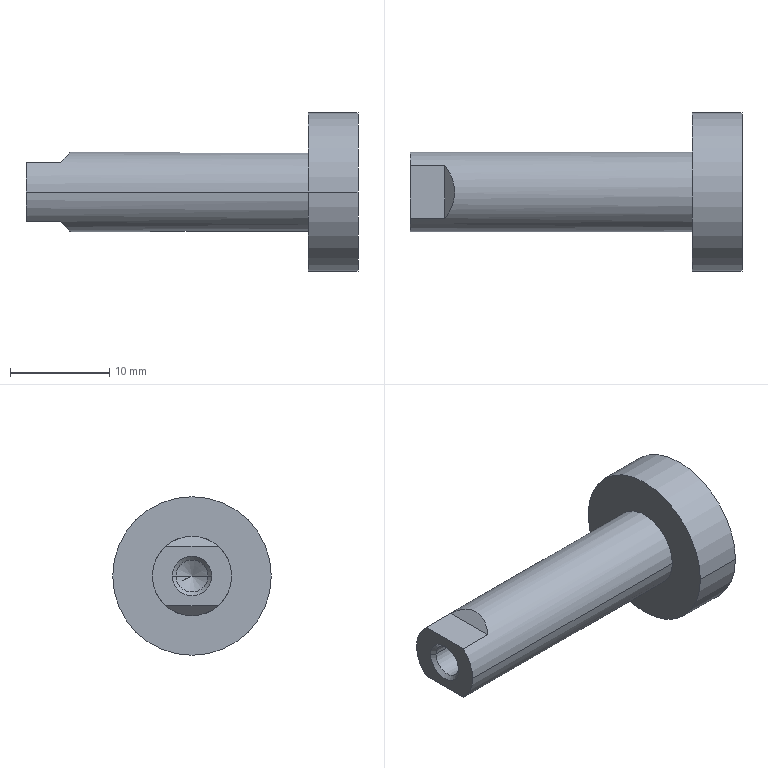Part | SolidWorks | features RefAxis 3, 3DProfileFeature 1, ICE 1, Revolution 1 | 1 solid | 17 faces | box 33.5 x 16 x 16 mm | volume 2340 mm3 | plane 7 | cylinder 6 | cone 4 | commonest cylinder face diameters 3.242 x2 8 x2 16 x2
STEP:
#1=CARTESIAN_POINT('',(30.,-8.,0.));
#2=VERTEX_POINT('',#1);
#3=CARTESIAN_POINT('',(30.,8.,0.));
#4=VERTEX_POINT('',#3);
#5=CARTESIAN_POINT('',(30.,0.,0.));
#6=DIRECTION('',(-1.,0.,0.));
#7=DIRECTION('',(0.,-1.,0.));
#8=AXIS2_PLACEMENT_3D('',#5,#6,#7);
#9=CIRCLE('',#8,8.);
#10=EDGE_CURVE('',#2,#4,#9,.T.);
#11=ORIENTED_EDGE('',*,*,#10,.T.);
#12=CARTESIAN_POINT('',(25.,8.,0.));
#13=VERTEX_POINT('',#12);
#14=CARTESIAN_POINT('',(30.,8.,0.));
#15=DIRECTION('',(-1.,0.,0.));
#16=VECTOR('',#15,1000.);
#17=LINE('',#14,#16);
#18=EDGE_CURVE('',#4,#13,#17,.T.);
#19=ORIENTED_EDGE('',*,*,#18,.T.);
#20=CARTESIAN_POINT('',(25.,-8.,0.));
#21=VERTEX_POINT('',#20);
#22=CARTESIAN_POINT('',(25.,0.,0.));
#23=DIRECTION('',(-1.,0.,0.));
#24=DIRECTION('',(0.,-1.,0.));
#25=AXIS2_PLACEMENT_3D('',#22,#23,#24);
#26=CIRCLE('',#25,8.);
#27=EDGE_CURVE('',#21,#13,#26,.T.);
#28=ORIENTED_EDGE('',*,*,#27,.F.);
#29=CARTESIAN_POINT('',(30.,-8.,0.));
#30=DIRECTION('',(-1.,0.,0.));
#31=VECTOR('',#30,1000.);
#32=LINE('',#29,#31);
#33=EDGE_CURVE('',#2,#21,#32,.T.);
#34=ORIENTED_EDGE('',*,*,#33,.F.);
#35=EDGE_LOOP('',(#11,#19,#28,#34));
#36=FACE_OUTER_BOUND('',#35,.T.);
#37=CARTESIAN_POINT('',(30.,0.,0.));
#38=DIRECTION('',(-1.,0.,0.));
#39=DIRECTION('',(0.,-1.,0.));
#40=AXIS2_PLACEMENT_3D('',#37,#38,#39);
#41=CYLINDRICAL_SURFACE('',#40,8.);
#42=ADVANCED_FACE('',(#36),#41,.T.);
#43=CARTESIAN_POINT('',(25.,-4.,0.));
#44=VERTEX_POINT('',#43);
#45=CARTESIAN_POINT('',(25.,4.,0.));
#46=VERTEX_POINT('',#45);
#47=CARTESIAN_POINT('',(25.,0.,0.));
#48=DIRECTION('',(-1.,0.,0.));
#49=DIRECTION('',(0.,-1.,0.));
#50=AXIS2_PLACEMENT_3D('',#47,#48,#49);
#51=CIRCLE('',#50,4.);
#52=EDGE_CURVE('',#44,#46,#51,.T.);
#53=ORIENTED_EDGE('',*,*,#52,.T.);
#54=CARTESIAN_POINT('',(-3.5,4.,0.));
#55=VERTEX_POINT('',#54);
#56=CARTESIAN_POINT('',(30.,4.,0.));
#57=DIRECTION('',(-1.,0.,0.));
#58=VECTOR('',#57,1000.);
#59=LINE('',#56,#58);
#60=EDGE_CURVE('',#46,#55,#59,.T.);
#61=ORIENTED_EDGE('',*,*,#60,.T.);
#62=CARTESIAN_POINT('',(-3.5,2.646,3.));
#63=VERTEX_POINT('',#62);
#64=CARTESIAN_POINT('',(-3.5,0.,0.));
#65=DIRECTION('',(-1.,0.,0.));
#66=DIRECTION('',(0.,-1.,0.));
#67=AXIS2_PLACEMENT_3D('',#64,#65,#66);
#68=CIRCLE('',#67,4.);
#69=EDGE_CURVE('',#63,#55,#68,.T.);
#70=ORIENTED_EDGE('',*,*,#69,.F.);
#71=CARTESIAN_POINT('',(0.,2.646,3.));
#72=VERTEX_POINT('',#71);
#73=CARTESIAN_POINT('',(30.,2.646,3.));
#74=DIRECTION('',(1.,0.,0.));
#75=VECTOR('',#74,1000.);
#76=LINE('',#73,#75);
#77=EDGE_CURVE('',#63,#72,#76,.T.);
#78=ORIENTED_EDGE('',*,*,#77,.T.);
#79=CARTESIAN_POINT('',(0.,-2.646,3.));
#80=VERTEX_POINT('',#79);
#81=CARTESIAN_POINT('',(0.,2.646,3.));
#82=CARTESIAN_POINT('',(1.4,1.058,4.4));
#83=CARTESIAN_POINT('',(1.4,-1.058,4.4));
#84=CARTESIAN_POINT('',(0.,-2.646,3.));
#85=(BOUNDED_CURVE()B_SPLINE_CURVE(3,(#81,#82,#83,#84),.UNSPECIFIED.,.F.,.T.)B_SPLINE_CURVE_WITH_KNOTS((4,4),(2.419,3.864),.UNSPECIFIED.)CURVE()GEOMETRIC_REPRESENTATION_ITEM()RATIONAL_B_SPLINE_CURVE((1.,0.8333,0.8333,1.))REPRESENTATION_ITEM(''));
#86=EDGE_CURVE('',#72,#80,#85,.T.);
#87=ORIENTED_EDGE('',*,*,#86,.T.);
#88=CARTESIAN_POINT('',(-3.5,-2.646,3.));
#89=VERTEX_POINT('',#88);
#90=CARTESIAN_POINT('',(30.,-2.646,3.));
#91=DIRECTION('',(-1.,0.,0.));
#92=VECTOR('',#91,1000.);
#93=LINE('',#90,#92);
#94=EDGE_CURVE('',#80,#89,#93,.T.);
#95=ORIENTED_EDGE('',*,*,#94,.T.);
#96=CARTESIAN_POINT('',(-3.5,-4.,0.));
#97=VERTEX_POINT('',#96);
#98=CARTESIAN_POINT('',(-3.5,0.,0.));
#99=DIRECTION('',(-1.,0.,0.));
#100=DIRECTION('',(0.,-1.,0.));
#101=AXIS2_PLACEMENT_3D('',#98,#99,#100);
#102=CIRCLE('',#101,4.);
#103=EDGE_CURVE('',#97,#89,#102,.T.);
#104=ORIENTED_EDGE('',*,*,#103,.F.);
#105=CARTESIAN_POINT('',(30.,-4.,0.));
#106=DIRECTION('',(-1.,0.,0.));
#107=VECTOR('',#106,1000.);
#108=LINE('',#105,#107);
#109=EDGE_CURVE('',#44,#97,#108,.T.);
#110=ORIENTED_EDGE('',*,*,#109,.F.);
#111=EDGE_LOOP('',(#53,#61,#70,#78,#87,#95,#104,#110));
#112=FACE_OUTER_BOUND('',#111,.T.);
#113=CARTESIAN_POINT('',(30.,0.,0.));
#114=DIRECTION('',(-1.,0.,0.));
#115=DIRECTION('',(0.,-1.,0.));
#116=AXIS2_PLACEMENT_3D('',#113,#114,#115);
#117=CYLINDRICAL_SURFACE('',#116,4.);
#118=ADVANCED_FACE('',(#112),#117,.T.);
#119=CARTESIAN_POINT('',(-3.121,1.621,0.));
#120=VERTEX_POINT('',#119);
#121=CARTESIAN_POINT('',(-3.121,-1.621,0.));
#122=VERTEX_POINT('',#121);
#123=CARTESIAN_POINT('',(-3.121,0.,0.));
#124=DIRECTION('',(-1.,0.,0.));
#125=DIRECTION('',(0.,-1.,0.));
#126=AXIS2_PLACEMENT_3D('',#123,#124,#125);
#127=CIRCLE('',#126,1.621);
#128=EDGE_CURVE('',#120,#122,#127,.T.);
#129=ORIENTED_EDGE('',*,*,#128,.F.);
#130=CARTESIAN_POINT('',(-3.5,2.,0.));
#131=VERTEX_POINT('',#130);
#132=CARTESIAN_POINT('',(-3.5,2.,0.));
#133=DIRECTION('',(-0.7071,0.7071,0.));
#134=VECTOR('',#133,1000.);
#135=LINE('',#132,#134);
#136=EDGE_CURVE('',#120,#131,#135,.T.);
#137=ORIENTED_EDGE('',*,*,#136,.T.);
#138=CARTESIAN_POINT('',(-3.5,-2.,0.));
#139=VERTEX_POINT('',#138);
#140=CARTESIAN_POINT('',(-3.5,0.,0.));
#141=DIRECTION('',(-1.,0.,0.));
#142=DIRECTION('',(0.,-1.,0.));
#143=AXIS2_PLACEMENT_3D('',#140,#141,#142);
#144=CIRCLE('',#143,2.);
#145=EDGE_CURVE('',#131,#139,#144,.T.);
#146=ORIENTED_EDGE('',*,*,#145,.T.);
#147=CARTESIAN_POINT('',(-3.5,-2.,0.));
#148=DIRECTION('',(-0.7071,-0.7071,0.));
#149=VECTOR('',#148,1000.);
#150=LINE('',#147,#149);
#151=EDGE_CURVE('',#122,#139,#150,.T.);
#152=ORIENTED_EDGE('',*,*,#151,.F.);
#153=EDGE_LOOP('',(#129,#137,#146,#152));
#154=FACE_OUTER_BOUND('',#153,.T.);
#155=CARTESIAN_POINT('',(-3.5,0.,0.));
#156=DIRECTION('',(-1.,0.,0.));
#157=DIRECTION('',(0.,-1.,0.));
#158=AXIS2_PLACEMENT_3D('',#155,#156,#157);
#159=CONICAL_SURFACE('',#158,2.,0.7854);
#160=ADVANCED_FACE('',(#154),#159,.F.);
#161=CARTESIAN_POINT('',(4.5,1.621,0.));
#162=VERTEX_POINT('',#161);
#163=CARTESIAN_POINT('',(4.5,-1.621,0.));
#164=VERTEX_POINT('',#163);
#165=CARTESIAN_POINT('',(4.5,0.,0.));
#166=DIRECTION('',(-1.,0.,0.));
#167=DIRECTION('',(0.,-1.,0.));
#168=AXIS2_PLACEMENT_3D('',#165,#166,#167);
#169=CIRCLE('',#168,1.621);
#170=EDGE_CURVE('',#162,#164,#169,.T.);
#171=ORIENTED_EDGE('',*,*,#170,.F.);
#172=CARTESIAN_POINT('',(30.,1.621,0.));
#173=DIRECTION('',(-1.,0.,0.));
#174=VECTOR('',#173,1000.);
#175=LINE('',#172,#174);
#176=EDGE_CURVE('',#162,#120,#175,.T.);
#177=ORIENTED_EDGE('',*,*,#176,.T.);
#178=ORIENTED_EDGE('',*,*,#128,.T.);
#179=CARTESIAN_POINT('',(30.,-1.621,0.));
#180=DIRECTION('',(-1.,0.,0.));
#181=VECTOR('',#180,1000.);
#182=LINE('',#179,#181);
#183=EDGE_CURVE('',#164,#122,#182,.T.);
#184=ORIENTED_EDGE('',*,*,#183,.F.);
#185=EDGE_LOOP('',(#171,#177,#178,#184));
#186=FACE_OUTER_BOUND('',#185,.T.);
#187=CARTESIAN_POINT('',(30.,0.,0.));
#188=DIRECTION('',(-1.,0.,0.));
#189=DIRECTION('',(0.,-1.,0.));
#190=AXIS2_PLACEMENT_3D('',#187,#188,#189);
#191=CYLINDRICAL_SURFACE('',#190,1.621);
#192=ADVANCED_FACE('',(#186),#191,.F.);
#193=CARTESIAN_POINT('',(5.436,0.,0.));
#194=VERTEX_POINT('',#193);
#195=CARTESIAN_POINT('',(4.5,-1.621,0.));
#196=DIRECTION('',(-0.5,-0.866,0.));
#197=VECTOR('',#196,1000.);
#198=LINE('',#195,#197);
#199=EDGE_CURVE('',#194,#164,#198,.T.);
#200=ORIENTED_EDGE('',*,*,#199,.F.);
#201=CARTESIAN_POINT('',(4.5,1.621,0.));
#202=DIRECTION('',(-0.5,0.866,0.));
#203=VECTOR('',#202,1000.);
#204=LINE('',#201,#203);
#205=EDGE_CURVE('',#194,#162,#204,.T.);
#206=ORIENTED_EDGE('',*,*,#205,.T.);
#207=ORIENTED_EDGE('',*,*,#170,.T.);
#208=EDGE_LOOP('',(#200,#206,#207));
#209=FACE_OUTER_BOUND('',#208,.T.);
#210=CARTESIAN_POINT('',(4.5,0.,0.));
#211=DIRECTION('',(-1.,0.,0.));
#212=DIRECTION('',(0.,-1.,0.));
#213=AXIS2_PLACEMENT_3D('',#210,#211,#212);
#214=CONICAL_SURFACE('',#213,1.621,1.047);
#215=ADVANCED_FACE('',(#209),#214,.F.);
#216=ORIENTED_EDGE('',*,*,#205,.F.);
#217=ORIENTED_EDGE('',*,*,#199,.T.);
#218=CARTESIAN_POINT('',(4.5,0.,0.));
#219=DIRECTION('',(-1.,0.,0.));
#220=DIRECTION('',(0.,-1.,0.));
#221=AXIS2_PLACEMENT_3D('',#218,#219,#220);
#222=CIRCLE('',#221,1.621);
#223=EDGE_CURVE('',#164,#162,#222,.T.);
#224=ORIENTED_EDGE('',*,*,#223,.T.);
#225=EDGE_LOOP('',(#216,#217,#224));
#226=FACE_OUTER_BOUND('',#225,.T.);
#227=CARTESIAN_POINT('',(4.5,0.,0.));
#228=DIRECTION('',(-1.,0.,0.));
#229=DIRECTION('',(0.,-1.,0.));
#230=AXIS2_PLACEMENT_3D('',#227,#228,#229);
#231=CONICAL_SURFACE('',#230,1.621,1.047);
#232=ADVANCED_FACE('',(#226),#231,.F.);
#233=ORIENTED_EDGE('',*,*,#176,.F.);
#234=ORIENTED_EDGE('',*,*,#223,.F.);
#235=ORIENTED_EDGE('',*,*,#183,.T.);
#236=CARTESIAN_POINT('',(-3.121,0.,0.));
#237=DIRECTION('',(-1.,0.,0.));
#238=DIRECTION('',(0.,-1.,0.));
#239=AXIS2_PLACEMENT_3D('',#236,#237,#238);
#240=CIRCLE('',#239,1.621);
#241=EDGE_CURVE('',#122,#120,#240,.T.);
#242=ORIENTED_EDGE('',*,*,#241,.T.);
#243=EDGE_LOOP('',(#233,#234,#235,#242));
#244=FACE_OUTER_BOUND('',#243,.T.);
#245=CARTESIAN_POINT('',(30.,0.,0.));
#246=DIRECTION('',(-1.,0.,0.));
#247=DIRECTION('',(0.,-1.,0.));
#248=AXIS2_PLACEMENT_3D('',#245,#246,#247);
#249=CYLINDRICAL_SURFACE('',#248,1.621);
#250=ADVANCED_FACE('',(#244),#249,.F.);
#251=ORIENTED_EDGE('',*,*,#136,.F.);
#252=ORIENTED_EDGE('',*,*,#241,.F.);
#253=ORIENTED_EDGE('',*,*,#151,.T.);
#254=CARTESIAN_POINT('',(-3.5,0.,0.));
#255=DIRECTION('',(-1.,0.,0.));
#256=DIRECTION('',(0.,-1.,0.));
#257=AXIS2_PLACEMENT_3D('',#254,#255,#256);
#258=CIRCLE('',#257,2.);
#259=EDGE_CURVE('',#139,#131,#258,.T.);
#260=ORIENTED_EDGE('',*,*,#259,.T.);
#261=EDGE_LOOP('',(#251,#252,#253,#260));
#262=FACE_OUTER_BOUND('',#261,.T.);
#263=CARTESIAN_POINT('',(-3.5,0.,0.));
#264=DIRECTION('',(-1.,0.,0.));
#265=DIRECTION('',(0.,-1.,0.));
#266=AXIS2_PLACEMENT_3D('',#263,#264,#265);
#267=CONICAL_SURFACE('',#266,2.,0.7854);
#268=ADVANCED_FACE('',(#262),#267,.F.);
#269=ORIENTED_EDGE('',*,*,#259,.F.);
#270=ORIENTED_EDGE('',*,*,#145,.F.);
#271=EDGE_LOOP('',(#269,#270));
#272=FACE_BOUND('',#271,.T.);
#273=ORIENTED_EDGE('',*,*,#69,.T.);
#274=CARTESIAN_POINT('',(-3.5,2.646,-3.));
#275=VERTEX_POINT('',#274);
#276=CARTESIAN_POINT('',(-3.5,0.,0.));
#277=DIRECTION('',(-1.,0.,0.));
#278=DIRECTION('',(0.,-1.,0.));
#279=AXIS2_PLACEMENT_3D('',#276,#277,#278);
#280=CIRCLE('',#279,4.);
#281=EDGE_CURVE('',#55,#275,#280,.T.);
#282=ORIENTED_EDGE('',*,*,#281,.T.);
#283=CARTESIAN_POINT('',(-3.5,-2.646,-3.));
#284=VERTEX_POINT('',#283);
#285=CARTESIAN_POINT('',(-3.5,-8.,-3.));
#286=DIRECTION('',(0.,1.,0.));
#287=VECTOR('',#286,1000.);
#288=LINE('',#285,#287);
#289=EDGE_CURVE('',#284,#275,#288,.T.);
#290=ORIENTED_EDGE('',*,*,#289,.F.);
#291=CARTESIAN_POINT('',(-3.5,0.,0.));
#292=DIRECTION('',(-1.,0.,0.));
#293=DIRECTION('',(0.,-1.,0.));
#294=AXIS2_PLACEMENT_3D('',#291,#292,#293);
#295=CIRCLE('',#294,4.);
#296=EDGE_CURVE('',#284,#97,#295,.T.);
#297=ORIENTED_EDGE('',*,*,#296,.T.);
#298=ORIENTED_EDGE('',*,*,#103,.T.);
#299=CARTESIAN_POINT('',(-3.5,-8.,3.));
#300=DIRECTION('',(0.,1.,0.));
#301=VECTOR('',#300,1000.);
#302=LINE('',#299,#301);
#303=EDGE_CURVE('',#89,#63,#302,.T.);
#304=ORIENTED_EDGE('',*,*,#303,.T.);
#305=EDGE_LOOP('',(#273,#282,#290,#297,#298,#304));
#306=FACE_OUTER_BOUND('',#305,.T.);
#307=CARTESIAN_POINT('',(-3.5,2.,0.));
#308=DIRECTION('',(1.,0.,0.));
#309=DIRECTION('',(0.,1.,0.));
#310=AXIS2_PLACEMENT_3D('',#307,#308,#309);
#311=PLANE('',#310);
#312=ADVANCED_FACE('',(#272,#306),#311,.F.);
#313=ORIENTED_EDGE('',*,*,#60,.F.);
#314=CARTESIAN_POINT('',(25.,0.,0.));
#315=DIRECTION('',(-1.,0.,0.));
#316=DIRECTION('',(0.,-1.,0.));
#317=AXIS2_PLACEMENT_3D('',#314,#315,#316);
#318=CIRCLE('',#317,4.);
#319=EDGE_CURVE('',#46,#44,#318,.T.);
#320=ORIENTED_EDGE('',*,*,#319,.T.);
#321=ORIENTED_EDGE('',*,*,#109,.T.);
#322=ORIENTED_EDGE('',*,*,#296,.F.);
#323=CARTESIAN_POINT('',(0.,-2.646,-3.));
#324=VERTEX_POINT('',#323);
#325=CARTESIAN_POINT('',(30.,-2.646,-3.));
#326=DIRECTION('',(1.,0.,0.));
#327=VECTOR('',#326,1000.);
#328=LINE('',#325,#327);
#329=EDGE_CURVE('',#284,#324,#328,.T.);
#330=ORIENTED_EDGE('',*,*,#329,.T.);
#331=CARTESIAN_POINT('',(0.,2.646,-3.));
#332=VERTEX_POINT('',#331);
#333=CARTESIAN_POINT('',(0.,-2.646,-3.));
#334=CARTESIAN_POINT('',(1.4,-1.058,-4.4));
#335=CARTESIAN_POINT('',(1.4,1.058,-4.4));
#336=CARTESIAN_POINT('',(0.,2.646,-3.));
#337=(BOUNDED_CURVE()B_SPLINE_CURVE(3,(#333,#334,#335,#336),.UNSPECIFIED.,.F.,.F.)B_SPLINE_CURVE_WITH_KNOTS((4,4),(2.419,3.864),.UNSPECIFIED.)CURVE()GEOMETRIC_REPRESENTATION_ITEM()RATIONAL_B_SPLINE_CURVE((1.,0.8333,0.8333,1.))REPRESENTATION_ITEM(''));
#338=EDGE_CURVE('',#324,#332,#337,.T.);
#339=ORIENTED_EDGE('',*,*,#338,.T.);
#340=CARTESIAN_POINT('',(30.,2.646,-3.));
#341=DIRECTION('',(-1.,0.,0.));
#342=VECTOR('',#341,1000.);
#343=LINE('',#340,#342);
#344=EDGE_CURVE('',#332,#275,#343,.T.);
#345=ORIENTED_EDGE('',*,*,#344,.T.);
#346=ORIENTED_EDGE('',*,*,#281,.F.);
#347=EDGE_LOOP('',(#313,#320,#321,#322,#330,#339,#345,#346));
#348=FACE_OUTER_BOUND('',#347,.T.);
#349=CARTESIAN_POINT('',(30.,0.,0.));
#350=DIRECTION('',(-1.,0.,0.));
#351=DIRECTION('',(0.,-1.,0.));
#352=AXIS2_PLACEMENT_3D('',#349,#350,#351);
#353=CYLINDRICAL_SURFACE('',#352,4.);
#354=ADVANCED_FACE('',(#348),#353,.T.);
#355=ORIENTED_EDGE('',*,*,#52,.F.);
#356=ORIENTED_EDGE('',*,*,#319,.F.);
#357=EDGE_LOOP('',(#355,#356));
#358=FACE_BOUND('',#357,.T.);
#359=ORIENTED_EDGE('',*,*,#27,.T.);
#360=CARTESIAN_POINT('',(25.,0.,0.));
#361=DIRECTION('',(-1.,0.,0.));
#362=DIRECTION('',(0.,-1.,0.));
#363=AXIS2_PLACEMENT_3D('',#360,#361,#362);
#364=CIRCLE('',#363,8.);
#365=EDGE_CURVE('',#13,#21,#364,.T.);
#366=ORIENTED_EDGE('',*,*,#365,.T.);
#367=EDGE_LOOP('',(#359,#366));
#368=FACE_OUTER_BOUND('',#367,.T.);
#369=CARTESIAN_POINT('',(25.,4.,0.));
#370=DIRECTION('',(1.,0.,0.));
#371=DIRECTION('',(0.,1.,0.));
#372=AXIS2_PLACEMENT_3D('',#369,#370,#371);
#373=PLANE('',#372);
#374=ADVANCED_FACE('',(#358,#368),#373,.F.);
#375=ORIENTED_EDGE('',*,*,#18,.F.);
#376=CARTESIAN_POINT('',(30.,0.,0.));
#377=DIRECTION('',(-1.,0.,0.));
#378=DIRECTION('',(0.,-1.,0.));
#379=AXIS2_PLACEMENT_3D('',#376,#377,#378);
#380=CIRCLE('',#379,8.);
#381=EDGE_CURVE('',#4,#2,#380,.T.);
#382=ORIENTED_EDGE('',*,*,#381,.T.);
#383=ORIENTED_EDGE('',*,*,#33,.T.);
#384=ORIENTED_EDGE('',*,*,#365,.F.);
#385=EDGE_LOOP('',(#375,#382,#383,#384));
#386=FACE_OUTER_BOUND('',#385,.T.);
#387=CARTESIAN_POINT('',(30.,0.,0.));
#388=DIRECTION('',(-1.,0.,0.));
#389=DIRECTION('',(0.,-1.,0.));
#390=AXIS2_PLACEMENT_3D('',#387,#388,#389);
#391=CYLINDRICAL_SURFACE('',#390,8.);
#392=ADVANCED_FACE('',(#386),#391,.T.);
#393=ORIENTED_EDGE('',*,*,#10,.F.);
#394=ORIENTED_EDGE('',*,*,#381,.F.);
#395=EDGE_LOOP('',(#393,#394));
#396=FACE_OUTER_BOUND('',#395,.T.);
#397=CARTESIAN_POINT('',(30.,8.,0.));
#398=DIRECTION('',(-1.,0.,0.));
#399=DIRECTION('',(0.,-1.,0.));
#400=AXIS2_PLACEMENT_3D('',#397,#398,#399);
#401=PLANE('',#400);
#402=ADVANCED_FACE('',(#396),#401,.F.);
#403=CARTESIAN_POINT('',(0.,-8.,3.));
#404=DIRECTION('',(0.,1.,0.));
#405=VECTOR('',#404,1000.);
#406=LINE('',#403,#405);
#407=EDGE_CURVE('',#80,#72,#406,.T.);
#408=ORIENTED_EDGE('',*,*,#407,.F.);
#409=ORIENTED_EDGE('',*,*,#86,.F.);
#410=EDGE_LOOP('',(#408,#409));
#411=FACE_OUTER_BOUND('',#410,.T.);
#412=CARTESIAN_POINT('',(5.,-8.,8.));
#413=DIRECTION('',(0.7071,0.,-0.7071));
#414=DIRECTION('',(-0.7071,0.,-0.7071));
#415=AXIS2_PLACEMENT_3D('',#412,#413,#414);
#416=PLANE('',#415);
#417=ADVANCED_FACE('',(#411),#416,.F.);
#418=ORIENTED_EDGE('',*,*,#407,.T.);
#419=ORIENTED_EDGE('',*,*,#77,.F.);
#420=ORIENTED_EDGE('',*,*,#303,.F.);
#421=ORIENTED_EDGE('',*,*,#94,.F.);
#422=EDGE_LOOP('',(#418,#419,#420,#421));
#423=FACE_OUTER_BOUND('',#422,.T.);
#424=CARTESIAN_POINT('',(0.,-8.,3.));
#425=DIRECTION('',(0.,0.,-1.));
#426=DIRECTION('',(-1.,0.,0.));
#427=AXIS2_PLACEMENT_3D('',#424,#425,#426);
#428=PLANE('',#427);
#429=ADVANCED_FACE('',(#423),#428,.F.);
#430=CARTESIAN_POINT('',(0.,-8.,-3.));
#431=DIRECTION('',(0.,1.,0.));
#432=VECTOR('',#431,1000.);
#433=LINE('',#430,#432);
#434=EDGE_CURVE('',#324,#332,#433,.T.);
#435=ORIENTED_EDGE('',*,*,#434,.T.);
#436=ORIENTED_EDGE('',*,*,#338,.F.);
#437=EDGE_LOOP('',(#435,#436));
#438=FACE_OUTER_BOUND('',#437,.T.);
#439=CARTESIAN_POINT('',(0.,-8.,-3.));
#440=DIRECTION('',(0.7071,0.,0.7071));
#441=DIRECTION('',(0.7071,0.,-0.7071));
#442=AXIS2_PLACEMENT_3D('',#439,#440,#441);
#443=PLANE('',#442);
#444=ADVANCED_FACE('',(#438),#443,.F.);
#445=ORIENTED_EDGE('',*,*,#434,.F.);
#446=ORIENTED_EDGE('',*,*,#329,.F.);
#447=ORIENTED_EDGE('',*,*,#289,.T.);
#448=ORIENTED_EDGE('',*,*,#344,.F.);
#449=EDGE_LOOP('',(#445,#446,#447,#448));
#450=FACE_OUTER_BOUND('',#449,.T.);
#451=CARTESIAN_POINT('',(-3.5,-8.,-3.));
#452=DIRECTION('',(0.,0.,1.));
#453=DIRECTION('',(1.,0.,0.));
#454=AXIS2_PLACEMENT_3D('',#451,#452,#453);
#455=PLANE('',#454);
#456=ADVANCED_FACE('',(#450),#455,.F.);
#457=CLOSED_SHELL('',(#42,#118,#160,#192,#215,#232,#250,#268,#312,#354,#374,#392,#402,#417,#429,#444,#456));
#458=MANIFOLD_SOLID_BREP('',#457);
#459=CARTESIAN_POINT('',(0.,0.,0.));
#460=DIRECTION('',(0.,0.,1.));
#461=DIRECTION('',(1.,0.,0.));
#462=AXIS2_PLACEMENT_3D('',#459,#460,#461);
#463=(LENGTH_UNIT()NAMED_UNIT(*)SI_UNIT(.MILLI.,.METRE.));
#464=UNCERTAINTY_MEASURE_WITH_UNIT(LENGTH_MEASURE(0.00001),#463,'','');
#465=(NAMED_UNIT(*)PLANE_ANGLE_UNIT()SI_UNIT($,.RADIAN.));
#466=(NAMED_UNIT(*)SI_UNIT($,.STERADIAN.)SOLID_ANGLE_UNIT());
#467=(GEOMETRIC_REPRESENTATION_CONTEXT(3)GLOBAL_UNCERTAINTY_ASSIGNED_CONTEXT((#464))GLOBAL_UNIT_ASSIGNED_CONTEXT((#463,#465,#466))REPRESENTATION_CONTEXT('',''));
#468=ADVANCED_BREP_SHAPE_REPRESENTATION('',(#458,#462),#467);